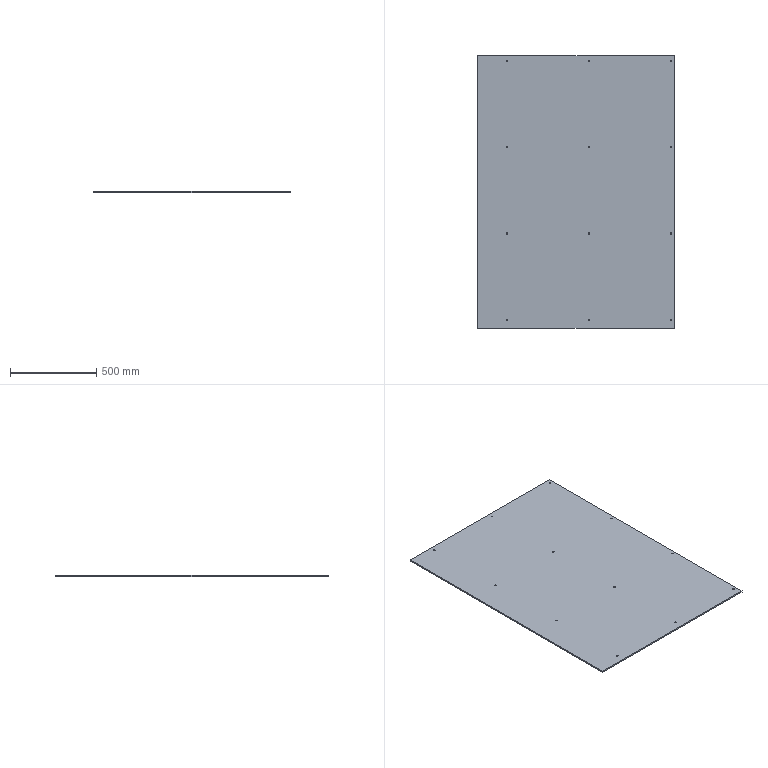Part | SolidWorks | features ICE 2, Extrusion 1 | 1 solid | 54 faces | box 1140 x 1580 x 8 mm | volume 14401036 mm3 | cone 24 | cylinder 24 | plane 6 | commonest cylinder face diameters 7 x24